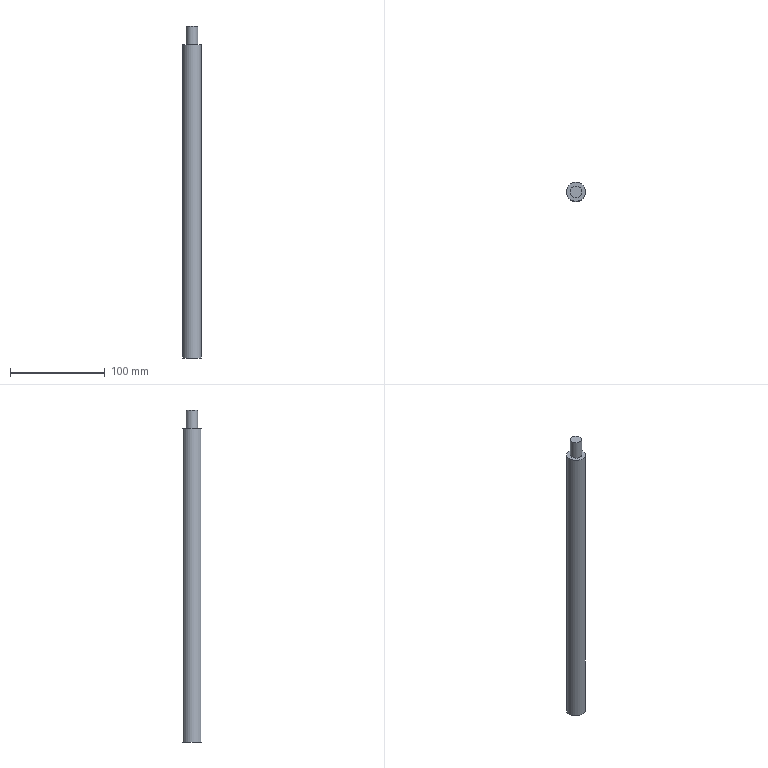Part | NX | features solid 2 | 1 solid | 7 faces | box 20 x 20 x 350 mm | volume 102406 mm3 | cylinder 3 | plane 3 | cone 1 | commonest cylinder face diameters 12 x2 20 x1
STEP:
#1=CARTESIAN_POINT('',(-745.,150.,70.));
#2=VERTEX_POINT('',#1);
#3=CARTESIAN_POINT('',(-735.,150.,70.));
#4=DIRECTION('',(0.,0.,-1.));
#5=DIRECTION('',(-1.,0.,0.));
#6=AXIS2_PLACEMENT_3D('',#3,#4,#5);
#7=CIRCLE('',#6,10.);
#8=EDGE_CURVE('',#2,#2,#7,.T.);
#9=ORIENTED_EDGE('',*,*,#8,.T.);
#10=EDGE_LOOP('',(#9));
#11=FACE_BOUND('',#10,.T.);
#12=CARTESIAN_POINT('',(-745.,150.,-260.));
#13=VERTEX_POINT('',#12);
#14=CARTESIAN_POINT('',(-735.,150.,-260.));
#15=DIRECTION('',(0.,0.,-1.));
#16=DIRECTION('',(-1.,0.,0.));
#17=AXIS2_PLACEMENT_3D('',#14,#15,#16);
#18=CIRCLE('',#17,10.);
#19=EDGE_CURVE('',#13,#13,#18,.T.);
#20=ORIENTED_EDGE('',*,*,#19,.F.);
#21=EDGE_LOOP('',(#20));
#22=FACE_BOUND('',#21,.T.);
#23=CARTESIAN_POINT('',(-735.,150.,120.));
#24=DIRECTION('',(0.,0.,-1.));
#25=DIRECTION('',(-1.,0.,0.));
#26=AXIS2_PLACEMENT_3D('',#23,#24,#25);
#27=CYLINDRICAL_SURFACE('',#26,10.);
#28=ADVANCED_FACE('',(#11,#22),#27,.T.);
#29=CARTESIAN_POINT('',(-741.,150.,70.));
#30=VERTEX_POINT('',#29);
#31=CARTESIAN_POINT('',(-735.,150.,70.));
#32=DIRECTION('',(0.,0.,-1.));
#33=DIRECTION('',(-1.,0.,0.));
#34=AXIS2_PLACEMENT_3D('',#31,#32,#33);
#35=CIRCLE('',#34,6.);
#36=EDGE_CURVE('',#30,#30,#35,.T.);
#37=ORIENTED_EDGE('',*,*,#36,.T.);
#38=EDGE_LOOP('',(#37));
#39=FACE_BOUND('',#38,.T.);
#40=ORIENTED_EDGE('',*,*,#8,.F.);
#41=EDGE_LOOP('',(#40));
#42=FACE_BOUND('',#41,.T.);
#43=CARTESIAN_POINT('',(-735.,150.,70.));
#44=DIRECTION('',(0.,0.,-1.));
#45=DIRECTION('',(-1.,0.,0.));
#46=AXIS2_PLACEMENT_3D('',#43,#44,#45);
#47=PLANE('',#46);
#48=ADVANCED_FACE('',(#39,#42),#47,.F.);
#49=CARTESIAN_POINT('',(-729.,150.,-260.));
#50=VERTEX_POINT('',#49);
#51=CARTESIAN_POINT('',(-735.,150.,-260.));
#52=DIRECTION('',(0.,0.,1.));
#53=DIRECTION('',(1.,0.,0.));
#54=AXIS2_PLACEMENT_3D('',#51,#52,#53);
#55=CIRCLE('',#54,6.);
#56=EDGE_CURVE('',#50,#50,#55,.T.);
#57=ORIENTED_EDGE('',*,*,#56,.T.);
#58=EDGE_LOOP('',(#57));
#59=FACE_BOUND('',#58,.T.);
#60=ORIENTED_EDGE('',*,*,#19,.T.);
#61=EDGE_LOOP('',(#60));
#62=FACE_BOUND('',#61,.T.);
#63=CARTESIAN_POINT('',(-735.,150.,-260.));
#64=DIRECTION('',(0.,0.,-1.));
#65=DIRECTION('',(-1.,0.,0.));
#66=AXIS2_PLACEMENT_3D('',#63,#64,#65);
#67=PLANE('',#66);
#68=ADVANCED_FACE('',(#59,#62),#67,.T.);
#69=CARTESIAN_POINT('',(-729.,150.,-230.));
#70=VERTEX_POINT('',#69);
#71=CARTESIAN_POINT('',(-735.,150.,-230.));
#72=DIRECTION('',(0.,0.,1.));
#73=DIRECTION('',(1.,0.,0.));
#74=AXIS2_PLACEMENT_3D('',#71,#72,#73);
#75=CIRCLE('',#74,6.);
#76=EDGE_CURVE('',#70,#70,#75,.T.);
#77=ORIENTED_EDGE('',*,*,#76,.F.);
#78=EDGE_LOOP('',(#77));
#79=FACE_BOUND('',#78,.T.);
#80=CARTESIAN_POINT('',(-735.,150.,-226.395));
#81=VERTEX_POINT('',#80);
#82=VERTEX_LOOP('',#81);
#83=FACE_BOUND('',#82,.T.);
#84=CARTESIAN_POINT('',(-735.,150.,-230.));
#85=DIRECTION('',(0.,0.,-1.));
#86=DIRECTION('',(-1.,0.,0.));
#87=AXIS2_PLACEMENT_3D('',#84,#85,#86);
#88=CONICAL_SURFACE('',#87,6.,1.03);
#89=ADVANCED_FACE('',(#79,#83),#88,.F.);
#90=ORIENTED_EDGE('',*,*,#76,.T.);
#91=EDGE_LOOP('',(#90));
#92=FACE_BOUND('',#91,.T.);
#93=ORIENTED_EDGE('',*,*,#56,.F.);
#94=EDGE_LOOP('',(#93));
#95=FACE_BOUND('',#94,.T.);
#96=CARTESIAN_POINT('',(-735.,150.,-260.));
#97=DIRECTION('',(0.,0.,1.));
#98=DIRECTION('',(1.,0.,0.));
#99=AXIS2_PLACEMENT_3D('',#96,#97,#98);
#100=CYLINDRICAL_SURFACE('',#99,6.);
#101=ADVANCED_FACE('',(#92,#95),#100,.F.);
#102=CARTESIAN_POINT('',(-741.,150.,90.));
#103=VERTEX_POINT('',#102);
#104=CARTESIAN_POINT('',(-735.,150.,90.));
#105=DIRECTION('',(0.,0.,-1.));
#106=DIRECTION('',(-1.,0.,0.));
#107=AXIS2_PLACEMENT_3D('',#104,#105,#106);
#108=CIRCLE('',#107,6.);
#109=EDGE_CURVE('',#103,#103,#108,.T.);
#110=ORIENTED_EDGE('',*,*,#109,.T.);
#111=EDGE_LOOP('',(#110));
#112=FACE_BOUND('',#111,.T.);
#113=ORIENTED_EDGE('',*,*,#36,.F.);
#114=EDGE_LOOP('',(#113));
#115=FACE_BOUND('',#114,.T.);
#116=CARTESIAN_POINT('',(-735.,150.,90.));
#117=DIRECTION('',(0.,0.,-1.));
#118=DIRECTION('',(-1.,0.,0.));
#119=AXIS2_PLACEMENT_3D('',#116,#117,#118);
#120=CYLINDRICAL_SURFACE('',#119,6.);
#121=ADVANCED_FACE('',(#112,#115),#120,.T.);
#122=ORIENTED_EDGE('',*,*,#109,.F.);
#123=EDGE_LOOP('',(#122));
#124=FACE_BOUND('',#123,.T.);
#125=CARTESIAN_POINT('',(-735.,150.,90.));
#126=DIRECTION('',(0.,0.,-1.));
#127=DIRECTION('',(-1.,0.,0.));
#128=AXIS2_PLACEMENT_3D('',#125,#126,#127);
#129=PLANE('',#128);
#130=ADVANCED_FACE('',(#124),#129,.F.);
#131=CLOSED_SHELL('',(#28,#48,#68,#89,#101,#121,#130));
#132=MANIFOLD_SOLID_BREP('',#131);
#133=(LENGTH_UNIT()NAMED_UNIT(*)SI_UNIT(.MILLI.,.METRE.));
#134=UNCERTAINTY_MEASURE_WITH_UNIT(LENGTH_MEASURE(0.00001),#133,'','');
#135=(NAMED_UNIT(*)PLANE_ANGLE_UNIT()SI_UNIT($,.RADIAN.));
#136=(NAMED_UNIT(*)SI_UNIT($,.STERADIAN.)SOLID_ANGLE_UNIT());
#137=(GEOMETRIC_REPRESENTATION_CONTEXT(3)GLOBAL_UNCERTAINTY_ASSIGNED_CONTEXT((#134))GLOBAL_UNIT_ASSIGNED_CONTEXT((#133,#135,#136))REPRESENTATION_CONTEXT('',''));
#138=ADVANCED_BREP_SHAPE_REPRESENTATION('',(#132),#137);